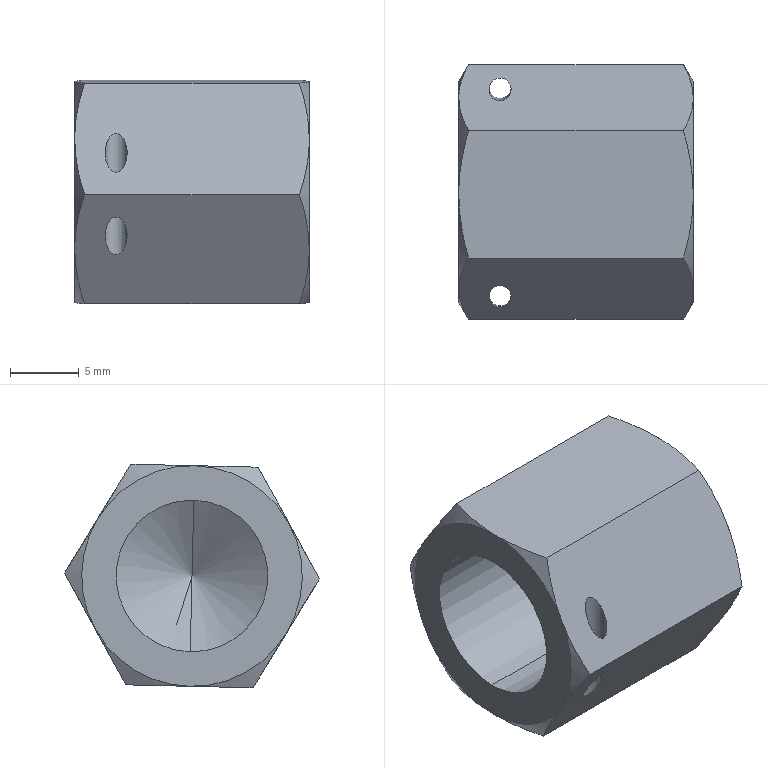Part | SolidWorks | features BaseBody 1 | 1 solid | 32 faces | box 17 x 18.47 x 16.209 mm | volume 2408 mm3 | cone 14 | plane 10 | cylinder 8 | commonest cylinder face diameters 1.6 x4 11 x2 12.5 x2
STEP:
#1=CARTESIAN_POINT('',(448.8,80.572,-3.182));
#2=VERTEX_POINT('',#1);
#3=CARTESIAN_POINT('',(450.4,80.572,-3.182));
#4=VERTEX_POINT('',#3);
#5=CARTESIAN_POINT('',(448.8,80.572,-3.182));
#6=CARTESIAN_POINT('',(448.8,78.908,-0.4485));
#7=CARTESIAN_POINT('',(450.4,78.908,-0.4485));
#8=CARTESIAN_POINT('',(450.4,80.572,-3.182));
#9=(BOUNDED_CURVE()B_SPLINE_CURVE(3,(#5,#6,#7,#8),.UNSPECIFIED.,.F.,.T.)B_SPLINE_CURVE_WITH_KNOTS((4,4),(4.712,7.854),.UNSPECIFIED.)CURVE()GEOMETRIC_REPRESENTATION_ITEM()RATIONAL_B_SPLINE_CURVE((1.,0.3333,0.3333,1.))REPRESENTATION_ITEM(''));
#10=EDGE_CURVE('',#2,#4,#9,.T.);
#11=ORIENTED_EDGE('',*,*,#10,.F.);
#12=CARTESIAN_POINT('',(448.8,80.432,2.836));
#13=VERTEX_POINT('',#12);
#14=CARTESIAN_POINT('',(448.8,80.687,-8.171));
#15=DIRECTION('',(0.,-0.0231,0.9997));
#16=VECTOR('',#15,1000.);
#17=LINE('',#14,#16);
#18=EDGE_CURVE('',#2,#13,#17,.T.);
#19=ORIENTED_EDGE('',*,*,#18,.T.);
#20=CARTESIAN_POINT('',(450.4,80.432,2.836));
#21=VERTEX_POINT('',#20);
#22=CARTESIAN_POINT('',(450.4,80.432,2.836));
#23=CARTESIAN_POINT('',(450.4,78.897,0.02809));
#24=CARTESIAN_POINT('',(448.8,78.897,0.02809));
#25=CARTESIAN_POINT('',(448.8,80.432,2.836));
#26=(BOUNDED_CURVE()B_SPLINE_CURVE(3,(#22,#23,#24,#25),.UNSPECIFIED.,.F.,.T.)B_SPLINE_CURVE_WITH_KNOTS((4,4),(1.571,4.712),.UNSPECIFIED.)CURVE()GEOMETRIC_REPRESENTATION_ITEM()RATIONAL_B_SPLINE_CURVE((1.,0.3333,0.3333,1.))REPRESENTATION_ITEM(''));
#27=EDGE_CURVE('',#21,#13,#26,.T.);
#28=ORIENTED_EDGE('',*,*,#27,.F.);
#29=CARTESIAN_POINT('',(450.4,80.687,-8.171));
#30=DIRECTION('',(0.,-0.0231,0.9997));
#31=VECTOR('',#30,1000.);
#32=LINE('',#29,#31);
#33=EDGE_CURVE('',#4,#21,#32,.T.);
#34=ORIENTED_EDGE('',*,*,#33,.F.);
#35=EDGE_LOOP('',(#11,#19,#28,#34));
#36=FACE_OUTER_BOUND('',#35,.T.);
#37=CARTESIAN_POINT('',(449.6,80.687,-8.171));
#38=DIRECTION('',(0.,-0.0231,0.9997));
#39=DIRECTION('',(1.,0.,0.));
#40=AXIS2_PLACEMENT_3D('',#37,#38,#39);
#41=CYLINDRICAL_SURFACE('',#40,0.8);
#42=ADVANCED_FACE('',(#36),#41,.F.);
#43=CARTESIAN_POINT('',(448.8,95.568,-2.836));
#44=VERTEX_POINT('',#43);
#45=CARTESIAN_POINT('',(450.4,95.568,-2.836));
#46=VERTEX_POINT('',#45);
#47=CARTESIAN_POINT('',(448.8,95.568,-2.836));
#48=CARTESIAN_POINT('',(448.8,94.032,-5.643));
#49=CARTESIAN_POINT('',(450.4,94.032,-5.643));
#50=CARTESIAN_POINT('',(450.4,95.568,-2.836));
#51=(BOUNDED_CURVE()B_SPLINE_CURVE(3,(#47,#48,#49,#50),.UNSPECIFIED.,.F.,.T.)B_SPLINE_CURVE_WITH_KNOTS((4,4),(1.571,4.712),.UNSPECIFIED.)CURVE()GEOMETRIC_REPRESENTATION_ITEM()RATIONAL_B_SPLINE_CURVE((1.,0.3333,0.3333,1.))REPRESENTATION_ITEM(''));
#52=EDGE_CURVE('',#44,#46,#51,.T.);
#53=ORIENTED_EDGE('',*,*,#52,.F.);
#54=CARTESIAN_POINT('',(448.8,95.428,3.182));
#55=VERTEX_POINT('',#54);
#56=CARTESIAN_POINT('',(448.8,95.683,-7.825));
#57=DIRECTION('',(0.,-0.0231,0.9997));
#58=VECTOR('',#57,1000.);
#59=LINE('',#56,#58);
#60=EDGE_CURVE('',#44,#55,#59,.T.);
#61=ORIENTED_EDGE('',*,*,#60,.T.);
#62=CARTESIAN_POINT('',(450.4,95.428,3.182));
#63=VERTEX_POINT('',#62);
#64=CARTESIAN_POINT('',(450.4,95.428,3.182));
#65=CARTESIAN_POINT('',(450.4,93.765,5.916));
#66=CARTESIAN_POINT('',(448.8,93.765,5.916));
#67=CARTESIAN_POINT('',(448.8,95.428,3.182));
#68=(BOUNDED_CURVE()B_SPLINE_CURVE(3,(#64,#65,#66,#67),.UNSPECIFIED.,.F.,.F.)B_SPLINE_CURVE_WITH_KNOTS((4,4),(4.712,7.854),.UNSPECIFIED.)CURVE()GEOMETRIC_REPRESENTATION_ITEM()RATIONAL_B_SPLINE_CURVE((1.,0.3333,0.3333,1.))REPRESENTATION_ITEM(''));
#69=EDGE_CURVE('',#63,#55,#68,.T.);
#70=ORIENTED_EDGE('',*,*,#69,.F.);
#71=CARTESIAN_POINT('',(450.4,95.683,-7.825));
#72=DIRECTION('',(0.,-0.0231,0.9997));
#73=VECTOR('',#72,1000.);
#74=LINE('',#71,#73);
#75=EDGE_CURVE('',#46,#63,#74,.T.);
#76=ORIENTED_EDGE('',*,*,#75,.F.);
#77=EDGE_LOOP('',(#53,#61,#70,#76));
#78=FACE_OUTER_BOUND('',#77,.T.);
#79=CARTESIAN_POINT('',(449.6,95.683,-7.825));
#80=DIRECTION('',(0.,-0.0231,0.9997));
#81=DIRECTION('',(1.,0.,0.));
#82=AXIS2_PLACEMENT_3D('',#79,#80,#81);
#83=CYLINDRICAL_SURFACE('',#82,0.8);
#84=ADVANCED_FACE('',(#78),#83,.F.);
#85=CARTESIAN_POINT('',(461.905,88.,0.));
#86=VERTEX_POINT('',#85);
#87=CARTESIAN_POINT('',(458.6,87.873,5.499));
#88=VERTEX_POINT('',#87);
#89=CARTESIAN_POINT('',(458.6,87.873,5.499));
#90=DIRECTION('',(-0.515,-0.0198,0.8569));
#91=VECTOR('',#90,1000.);
#92=LINE('',#89,#91);
#93=EDGE_CURVE('',#86,#88,#92,.T.);
#94=ORIENTED_EDGE('',*,*,#93,.F.);
#95=CARTESIAN_POINT('',(458.6,88.127,-5.499));
#96=VERTEX_POINT('',#95);
#97=CARTESIAN_POINT('',(458.6,88.127,-5.499));
#98=DIRECTION('',(-0.515,0.0198,-0.8569));
#99=VECTOR('',#98,1000.);
#100=LINE('',#97,#99);
#101=EDGE_CURVE('',#86,#96,#100,.T.);
#102=ORIENTED_EDGE('',*,*,#101,.T.);
#103=CARTESIAN_POINT('',(458.6,88.,0.));
#104=DIRECTION('',(-1.,0.,0.));
#105=DIRECTION('',(0.,-0.0231,0.9997));
#106=AXIS2_PLACEMENT_3D('',#103,#104,#105);
#107=CIRCLE('',#106,5.5);
#108=EDGE_CURVE('',#96,#88,#107,.T.);
#109=ORIENTED_EDGE('',*,*,#108,.T.);
#110=EDGE_LOOP('',(#94,#102,#109));
#111=FACE_OUTER_BOUND('',#110,.T.);
#112=CARTESIAN_POINT('',(458.6,88.,0.));
#113=DIRECTION('',(-1.,0.,0.));
#114=DIRECTION('',(0.,-0.0231,0.9997));
#115=AXIS2_PLACEMENT_3D('',#112,#113,#114);
#116=CONICAL_SURFACE('',#115,5.5,1.03);
#117=ADVANCED_FACE('',(#111),#116,.F.);
#118=CARTESIAN_POINT('',(455.6,88.144,-6.248));
#119=VERTEX_POINT('',#118);
#120=CARTESIAN_POINT('',(455.6,87.856,6.248));
#121=VERTEX_POINT('',#120);
#122=CARTESIAN_POINT('',(455.6,88.,0.));
#123=DIRECTION('',(-1.,0.,0.));
#124=DIRECTION('',(0.,-0.0231,0.9997));
#125=AXIS2_PLACEMENT_3D('',#122,#123,#124);
#126=CIRCLE('',#125,6.25);
#127=EDGE_CURVE('',#119,#121,#126,.T.);
#128=ORIENTED_EDGE('',*,*,#127,.T.);
#129=CARTESIAN_POINT('',(458.6,87.856,6.248));
#130=VERTEX_POINT('',#129);
#131=CARTESIAN_POINT('',(455.6,87.856,6.248));
#132=DIRECTION('',(1.,0.,0.));
#133=VECTOR('',#132,1000.);
#134=LINE('',#131,#133);
#135=EDGE_CURVE('',#121,#130,#134,.T.);
#136=ORIENTED_EDGE('',*,*,#135,.T.);
#137=CARTESIAN_POINT('',(458.6,88.144,-6.248));
#138=VERTEX_POINT('',#137);
#139=CARTESIAN_POINT('',(458.6,88.,0.));
#140=DIRECTION('',(-1.,0.,0.));
#141=DIRECTION('',(0.,-0.0231,0.9997));
#142=AXIS2_PLACEMENT_3D('',#139,#140,#141);
#143=CIRCLE('',#142,6.25);
#144=EDGE_CURVE('',#138,#130,#143,.T.);
#145=ORIENTED_EDGE('',*,*,#144,.F.);
#146=CARTESIAN_POINT('',(455.6,88.144,-6.248));
#147=DIRECTION('',(1.,0.,0.));
#148=VECTOR('',#147,1000.);
#149=LINE('',#146,#148);
#150=EDGE_CURVE('',#119,#138,#149,.T.);
#151=ORIENTED_EDGE('',*,*,#150,.F.);
#152=EDGE_LOOP('',(#128,#136,#145,#151));
#153=FACE_OUTER_BOUND('',#152,.T.);
#154=CARTESIAN_POINT('',(455.6,88.,0.));
#155=DIRECTION('',(1.,0.,0.));
#156=DIRECTION('',(0.,0.0231,-0.9997));
#157=AXIS2_PLACEMENT_3D('',#154,#155,#156);
#158=CYLINDRICAL_SURFACE('',#157,6.25);
#159=ADVANCED_FACE('',(#153),#158,.F.);
#160=CARTESIAN_POINT('',(455.6,87.873,5.499));
#161=VERTEX_POINT('',#160);
#162=CARTESIAN_POINT('',(455.6,88.127,-5.499));
#163=VERTEX_POINT('',#162);
#164=CARTESIAN_POINT('',(455.6,88.,0.));
#165=DIRECTION('',(1.,0.,0.));
#166=DIRECTION('',(0.,-0.0231,0.9997));
#167=AXIS2_PLACEMENT_3D('',#164,#165,#166);
#168=CIRCLE('',#167,5.5);
#169=EDGE_CURVE('',#161,#163,#168,.T.);
#170=ORIENTED_EDGE('',*,*,#169,.T.);
#171=CARTESIAN_POINT('',(446.6,88.127,-5.499));
#172=VERTEX_POINT('',#171);
#173=CARTESIAN_POINT('',(458.6,88.127,-5.499));
#174=DIRECTION('',(-1.,0.,0.));
#175=VECTOR('',#174,1000.);
#176=LINE('',#173,#175);
#177=EDGE_CURVE('',#163,#172,#176,.T.);
#178=ORIENTED_EDGE('',*,*,#177,.T.);
#179=CARTESIAN_POINT('',(446.6,87.873,5.499));
#180=VERTEX_POINT('',#179);
#181=CARTESIAN_POINT('',(446.6,88.,0.));
#182=DIRECTION('',(-1.,0.,0.));
#183=DIRECTION('',(0.,-0.0231,0.9997));
#184=AXIS2_PLACEMENT_3D('',#181,#182,#183);
#185=CIRCLE('',#184,5.5);
#186=EDGE_CURVE('',#172,#180,#185,.T.);
#187=ORIENTED_EDGE('',*,*,#186,.T.);
#188=CARTESIAN_POINT('',(458.6,87.873,5.499));
#189=DIRECTION('',(-1.,0.,0.));
#190=VECTOR('',#189,1000.);
#191=LINE('',#188,#190);
#192=EDGE_CURVE('',#161,#180,#191,.T.);
#193=ORIENTED_EDGE('',*,*,#192,.F.);
#194=EDGE_LOOP('',(#170,#178,#187,#193));
#195=FACE_OUTER_BOUND('',#194,.T.);
#196=CARTESIAN_POINT('',(458.6,88.,0.));
#197=DIRECTION('',(-1.,0.,0.));
#198=DIRECTION('',(0.,-0.0231,0.9997));
#199=AXIS2_PLACEMENT_3D('',#196,#197,#198);
#200=CYLINDRICAL_SURFACE('',#199,5.5);
#201=ADVANCED_FACE('',(#195),#200,.F.);
#202=ORIENTED_EDGE('',*,*,#69,.T.);
#203=CARTESIAN_POINT('',(448.8,95.428,3.182));
#204=CARTESIAN_POINT('',(448.8,97.092,0.4485));
#205=CARTESIAN_POINT('',(450.4,97.092,0.4485));
#206=CARTESIAN_POINT('',(450.4,95.428,3.182));
#207=(BOUNDED_CURVE()B_SPLINE_CURVE(3,(#203,#204,#205,#206),.UNSPECIFIED.,.F.,.T.)B_SPLINE_CURVE_WITH_KNOTS((4,4),(1.571,4.712),.UNSPECIFIED.)CURVE()GEOMETRIC_REPRESENTATION_ITEM()RATIONAL_B_SPLINE_CURVE((1.,0.3333,0.3333,1.))REPRESENTATION_ITEM(''));
#208=EDGE_CURVE('',#55,#63,#207,.T.);
#209=ORIENTED_EDGE('',*,*,#208,.T.);
#210=EDGE_LOOP('',(#202,#209));
#211=FACE_BOUND('',#210,.T.);
#212=CARTESIAN_POINT('',(462.885,97.235,0.2134));
#213=VERTEX_POINT('',#212);
#214=CARTESIAN_POINT('',(463.6,94.834,4.159));
#215=VERTEX_POINT('',#214);
#216=CARTESIAN_POINT('',(462.885,97.235,0.2134));
#217=CARTESIAN_POINT('',(463.102,96.845,0.8545));
#218=CARTESIAN_POINT('',(463.282,96.451,1.502));
#219=CARTESIAN_POINT('',(463.469,95.851,2.487));
#220=CARTESIAN_POINT('',(463.517,95.65,2.818));
#221=CARTESIAN_POINT('',(463.583,95.244,3.485));
#222=CARTESIAN_POINT('',(463.6,95.039,3.823));
#223=CARTESIAN_POINT('',(463.6,94.834,4.159));
#224=B_SPLINE_CURVE_WITH_KNOTS('',3,(#216,#217,#218,#219,#220,#221,#222,#223),.UNSPECIFIED.,.F.,.F.,(4,2,2,4),(0.001304,0.003639,0.004807,0.005975),.UNSPECIFIED.);
#225=EDGE_CURVE('',#213,#215,#224,.T.);
#226=ORIENTED_EDGE('',*,*,#225,.F.);
#227=CARTESIAN_POINT('',(447.315,97.235,0.2134));
#228=VERTEX_POINT('',#227);
#229=CARTESIAN_POINT('',(446.6,97.235,0.2134));
#230=DIRECTION('',(1.,0.,0.));
#231=VECTOR('',#230,1000.);
#232=LINE('',#229,#231);
#233=EDGE_CURVE('',#228,#213,#232,.T.);
#234=ORIENTED_EDGE('',*,*,#233,.F.);
#235=CARTESIAN_POINT('',(446.6,94.834,4.159));
#236=VERTEX_POINT('',#235);
#237=CARTESIAN_POINT('',(446.6,94.834,4.159));
#238=CARTESIAN_POINT('',(446.6,95.039,3.823));
#239=CARTESIAN_POINT('',(446.617,95.244,3.485));
#240=CARTESIAN_POINT('',(446.683,95.65,2.818));
#241=CARTESIAN_POINT('',(446.731,95.851,2.487));
#242=CARTESIAN_POINT('',(446.918,96.451,1.502));
#243=CARTESIAN_POINT('',(447.098,96.845,0.8545));
#244=CARTESIAN_POINT('',(447.315,97.235,0.2134));
#245=B_SPLINE_CURVE_WITH_KNOTS('',3,(#237,#238,#239,#240,#241,#242,#243,#244),.UNSPECIFIED.,.F.,.F.,(4,2,2,4),(0.005009,0.006177,0.007344,0.009679),.UNSPECIFIED.);
#246=EDGE_CURVE('',#236,#228,#245,.T.);
#247=ORIENTED_EDGE('',*,*,#246,.F.);
#248=CARTESIAN_POINT('',(447.315,92.433,8.105));
#249=VERTEX_POINT('',#248);
#250=CARTESIAN_POINT('',(447.315,92.433,8.105));
#251=CARTESIAN_POINT('',(447.097,92.825,7.46));
#252=CARTESIAN_POINT('',(446.917,93.22,6.81));
#253=CARTESIAN_POINT('',(446.668,94.02,5.496));
#254=CARTESIAN_POINT('',(446.6,94.424,4.832));
#255=CARTESIAN_POINT('',(446.6,94.834,4.159));
#256=B_SPLINE_CURVE_WITH_KNOTS('',3,(#250,#251,#252,#253,#254,#255),.UNSPECIFIED.,.F.,.F.,(4,2,4),(0.0003354,0.002672,0.005009),.UNSPECIFIED.);
#257=EDGE_CURVE('',#249,#236,#256,.T.);
#258=ORIENTED_EDGE('',*,*,#257,.F.);
#259=CARTESIAN_POINT('',(462.885,92.433,8.105));
#260=VERTEX_POINT('',#259);
#261=CARTESIAN_POINT('',(446.6,92.433,8.105));
#262=DIRECTION('',(1.,0.,0.));
#263=VECTOR('',#262,1000.);
#264=LINE('',#261,#263);
#265=EDGE_CURVE('',#249,#260,#264,.T.);
#266=ORIENTED_EDGE('',*,*,#265,.T.);
#267=CARTESIAN_POINT('',(463.6,94.834,4.159));
#268=CARTESIAN_POINT('',(463.6,94.424,4.832));
#269=CARTESIAN_POINT('',(463.532,94.02,5.496));
#270=CARTESIAN_POINT('',(463.283,93.22,6.81));
#271=CARTESIAN_POINT('',(463.103,92.825,7.46));
#272=CARTESIAN_POINT('',(462.885,92.433,8.105));
#273=B_SPLINE_CURVE_WITH_KNOTS('',3,(#267,#268,#269,#270,#271,#272),.UNSPECIFIED.,.F.,.F.,(4,2,4),(0.005975,0.008312,0.01065),.UNSPECIFIED.);
#274=EDGE_CURVE('',#215,#260,#273,.T.);
#275=ORIENTED_EDGE('',*,*,#274,.F.);
#276=EDGE_LOOP('',(#226,#234,#247,#258,#266,#275));
#277=FACE_OUTER_BOUND('',#276,.T.);
#278=CARTESIAN_POINT('',(446.6,92.433,8.105));
#279=DIRECTION('',(0.,-0.8542,-0.5199));
#280=DIRECTION('',(0.,-0.5199,0.8542));
#281=AXIS2_PLACEMENT_3D('',#278,#279,#280);
#282=PLANE('',#281);
#283=ADVANCED_FACE('',(#211,#277),#282,.F.);
#284=CARTESIAN_POINT('',(450.4,95.568,-2.836));
#285=CARTESIAN_POINT('',(450.4,97.103,-0.02809));
#286=CARTESIAN_POINT('',(448.8,97.103,-0.02809));
#287=CARTESIAN_POINT('',(448.8,95.568,-2.836));
#288=(BOUNDED_CURVE()B_SPLINE_CURVE(3,(#284,#285,#286,#287),.UNSPECIFIED.,.F.,.F.)B_SPLINE_CURVE_WITH_KNOTS((4,4),(4.712,7.854),.UNSPECIFIED.)CURVE()GEOMETRIC_REPRESENTATION_ITEM()RATIONAL_B_SPLINE_CURVE((1.,0.3333,0.3333,1.))REPRESENTATION_ITEM(''));
#289=EDGE_CURVE('',#46,#44,#288,.T.);
#290=ORIENTED_EDGE('',*,*,#289,.T.);
#291=ORIENTED_EDGE('',*,*,#52,.T.);
#292=EDGE_LOOP('',(#290,#291));
#293=FACE_BOUND('',#292,.T.);
#294=CARTESIAN_POINT('',(462.885,92.802,-7.891));
#295=VERTEX_POINT('',#294);
#296=CARTESIAN_POINT('',(463.6,95.019,-3.839));
#297=VERTEX_POINT('',#296);
#298=CARTESIAN_POINT('',(462.885,92.802,-7.891));
#299=CARTESIAN_POINT('',(463.102,93.163,-7.232));
#300=CARTESIAN_POINT('',(463.284,93.532,-6.557));
#301=CARTESIAN_POINT('',(463.533,94.272,-5.204));
#302=CARTESIAN_POINT('',(463.6,94.644,-4.524));
#303=CARTESIAN_POINT('',(463.6,95.019,-3.839));
#304=B_SPLINE_CURVE_WITH_KNOTS('',3,(#298,#299,#300,#301,#302,#303),.UNSPECIFIED.,.F.,.F.,(4,2,4),(0.008227,0.01056,0.0129),.UNSPECIFIED.);
#305=EDGE_CURVE('',#295,#297,#304,.T.);
#306=ORIENTED_EDGE('',*,*,#305,.F.);
#307=CARTESIAN_POINT('',(447.315,92.802,-7.891));
#308=VERTEX_POINT('',#307);
#309=CARTESIAN_POINT('',(446.6,92.802,-7.891));
#310=DIRECTION('',(1.,0.,0.));
#311=VECTOR('',#310,1000.);
#312=LINE('',#309,#311);
#313=EDGE_CURVE('',#308,#295,#312,.T.);
#314=ORIENTED_EDGE('',*,*,#313,.F.);
#315=CARTESIAN_POINT('',(446.6,95.019,-3.839));
#316=VERTEX_POINT('',#315);
#317=CARTESIAN_POINT('',(446.6,95.019,-3.839));
#318=CARTESIAN_POINT('',(446.6,94.644,-4.524));
#319=CARTESIAN_POINT('',(446.667,94.272,-5.204));
#320=CARTESIAN_POINT('',(446.916,93.532,-6.557));
#321=CARTESIAN_POINT('',(447.098,93.163,-7.232));
#322=CARTESIAN_POINT('',(447.315,92.802,-7.891));
#323=B_SPLINE_CURVE_WITH_KNOTS('',3,(#317,#318,#319,#320,#321,#322),.UNSPECIFIED.,.F.,.F.,(4,2,4),(0.008064,0.01039,0.01272),.UNSPECIFIED.);
#324=EDGE_CURVE('',#316,#308,#323,.T.);
#325=ORIENTED_EDGE('',*,*,#324,.F.);
#326=CARTESIAN_POINT('',(447.315,97.235,0.2134));
#327=CARTESIAN_POINT('',(447.099,96.877,-0.4419));
#328=CARTESIAN_POINT('',(446.919,96.514,-1.106));
#329=CARTESIAN_POINT('',(446.669,95.773,-2.459));
#330=CARTESIAN_POINT('',(446.6,95.393,-3.154));
#331=CARTESIAN_POINT('',(446.6,95.019,-3.839));
#332=B_SPLINE_CURVE_WITH_KNOTS('',3,(#326,#327,#328,#329,#330,#331),.UNSPECIFIED.,.F.,.F.,(4,2,4),(0.003401,0.005732,0.008064),.UNSPECIFIED.);
#333=EDGE_CURVE('',#228,#316,#332,.T.);
#334=ORIENTED_EDGE('',*,*,#333,.F.);
#335=ORIENTED_EDGE('',*,*,#233,.T.);
#336=CARTESIAN_POINT('',(463.6,95.019,-3.839));
#337=CARTESIAN_POINT('',(463.6,95.393,-3.154));
#338=CARTESIAN_POINT('',(463.531,95.773,-2.459));
#339=CARTESIAN_POINT('',(463.281,96.514,-1.106));
#340=CARTESIAN_POINT('',(463.101,96.877,-0.4419));
#341=CARTESIAN_POINT('',(462.885,97.235,0.2134));
#342=B_SPLINE_CURVE_WITH_KNOTS('',3,(#336,#337,#338,#339,#340,#341),.UNSPECIFIED.,.F.,.F.,(4,2,4),(0.0129,0.01524,0.01757),.UNSPECIFIED.);
#343=EDGE_CURVE('',#297,#213,#342,.T.);
#344=ORIENTED_EDGE('',*,*,#343,.F.);
#345=EDGE_LOOP('',(#306,#314,#325,#334,#335,#344));
#346=FACE_OUTER_BOUND('',#345,.T.);
#347=CARTESIAN_POINT('',(446.6,97.235,0.2134));
#348=DIRECTION('',(0.,-0.8773,0.4799));
#349=DIRECTION('',(0.,0.4799,0.8773));
#350=AXIS2_PLACEMENT_3D('',#347,#348,#349);
#351=PLANE('',#350);
#352=ADVANCED_FACE('',(#293,#346),#351,.F.);
#353=CARTESIAN_POINT('',(462.885,83.567,-8.105));
#354=VERTEX_POINT('',#353);
#355=CARTESIAN_POINT('',(463.6,88.185,-7.998));
#356=VERTEX_POINT('',#355);
#357=CARTESIAN_POINT('',(462.885,83.567,-8.105));
#358=CARTESIAN_POINT('',(463.103,84.319,-8.087));
#359=CARTESIAN_POINT('',(463.284,85.088,-8.069));
#360=CARTESIAN_POINT('',(463.533,86.628,-8.034));
#361=CARTESIAN_POINT('',(463.6,87.403,-8.016));
#362=CARTESIAN_POINT('',(463.6,88.185,-7.998));
#363=B_SPLINE_CURVE_WITH_KNOTS('',3,(#357,#358,#359,#360,#361,#362),.UNSPECIFIED.,.F.,.F.,(4,2,4),(0.008667,0.01101,0.01334),.UNSPECIFIED.);
#364=EDGE_CURVE('',#354,#356,#363,.T.);
#365=ORIENTED_EDGE('',*,*,#364,.F.);
#366=CARTESIAN_POINT('',(447.315,83.567,-8.105));
#367=VERTEX_POINT('',#366);
#368=CARTESIAN_POINT('',(446.6,83.567,-8.105));
#369=DIRECTION('',(1.,0.,0.));
#370=VECTOR('',#369,1000.);
#371=LINE('',#368,#370);
#372=EDGE_CURVE('',#367,#354,#371,.T.);
#373=ORIENTED_EDGE('',*,*,#372,.F.);
#374=CARTESIAN_POINT('',(446.6,88.185,-7.998));
#375=VERTEX_POINT('',#374);
#376=CARTESIAN_POINT('',(446.6,88.185,-7.998));
#377=CARTESIAN_POINT('',(446.6,87.403,-8.016));
#378=CARTESIAN_POINT('',(446.667,86.628,-8.034));
#379=CARTESIAN_POINT('',(446.916,85.088,-8.069));
#380=CARTESIAN_POINT('',(447.097,84.319,-8.087));
#381=CARTESIAN_POINT('',(447.315,83.567,-8.105));
#382=B_SPLINE_CURVE_WITH_KNOTS('',3,(#376,#377,#378,#379,#380,#381),.UNSPECIFIED.,.F.,.F.,(4,2,4),(0.03992,0.04226,0.04459),.UNSPECIFIED.);
#383=EDGE_CURVE('',#375,#367,#382,.T.);
#384=ORIENTED_EDGE('',*,*,#383,.F.);
#385=CARTESIAN_POINT('',(447.315,92.802,-7.891));
#386=CARTESIAN_POINT('',(447.099,92.055,-7.908));
#387=CARTESIAN_POINT('',(446.919,91.299,-7.926));
#388=CARTESIAN_POINT('',(446.732,90.144,-7.953));
#389=CARTESIAN_POINT('',(446.683,89.755,-7.962));
#390=CARTESIAN_POINT('',(446.617,88.97,-7.98));
#391=CARTESIAN_POINT('',(446.6,88.576,-7.989));
#392=CARTESIAN_POINT('',(446.6,88.185,-7.998));
#393=B_SPLINE_CURVE_WITH_KNOTS('',3,(#385,#386,#387,#388,#389,#390,#391,#392),.UNSPECIFIED.,.F.,.F.,(4,2,2,4),(0.03525,0.03759,0.03875,0.03992),.UNSPECIFIED.);
#394=EDGE_CURVE('',#308,#375,#393,.T.);
#395=ORIENTED_EDGE('',*,*,#394,.F.);
#396=ORIENTED_EDGE('',*,*,#313,.T.);
#397=CARTESIAN_POINT('',(463.6,88.185,-7.998));
#398=CARTESIAN_POINT('',(463.6,88.576,-7.989));
#399=CARTESIAN_POINT('',(463.583,88.97,-7.98));
#400=CARTESIAN_POINT('',(463.517,89.755,-7.962));
#401=CARTESIAN_POINT('',(463.468,90.144,-7.953));
#402=CARTESIAN_POINT('',(463.281,91.299,-7.926));
#403=CARTESIAN_POINT('',(463.101,92.055,-7.908));
#404=CARTESIAN_POINT('',(462.885,92.802,-7.891));
#405=B_SPLINE_CURVE_WITH_KNOTS('',3,(#397,#398,#399,#400,#401,#402,#403,#404),.UNSPECIFIED.,.F.,.F.,(4,2,2,4),(0.01334,0.01451,0.01568,0.01802),.UNSPECIFIED.);
#406=EDGE_CURVE('',#356,#295,#405,.T.);
#407=ORIENTED_EDGE('',*,*,#406,.F.);
#408=EDGE_LOOP('',(#365,#373,#384,#395,#396,#407));
#409=FACE_OUTER_BOUND('',#408,.T.);
#410=CARTESIAN_POINT('',(446.6,92.802,-7.891));
#411=DIRECTION('',(0.,-0.0231,0.9997));
#412=DIRECTION('',(1.,0.,0.));
#413=AXIS2_PLACEMENT_3D('',#410,#411,#412);
#414=PLANE('',#413);
#415=ADVANCED_FACE('',(#409),#414,.F.);
#416=CARTESIAN_POINT('',(450.4,80.572,-3.182));
#417=CARTESIAN_POINT('',(450.4,82.235,-5.916));
#418=CARTESIAN_POINT('',(448.8,82.235,-5.916));
#419=CARTESIAN_POINT('',(448.8,80.572,-3.182));
#420=(BOUNDED_CURVE()B_SPLINE_CURVE(3,(#416,#417,#418,#419),.UNSPECIFIED.,.F.,.F.)B_SPLINE_CURVE_WITH_KNOTS((4,4),(1.571,4.712),.UNSPECIFIED.)CURVE()GEOMETRIC_REPRESENTATION_ITEM()RATIONAL_B_SPLINE_CURVE((1.,0.3333,0.3333,1.))REPRESENTATION_ITEM(''));
#421=EDGE_CURVE('',#4,#2,#420,.T.);
#422=ORIENTED_EDGE('',*,*,#421,.T.);
#423=ORIENTED_EDGE('',*,*,#10,.T.);
#424=EDGE_LOOP('',(#422,#423));
#425=FACE_BOUND('',#424,.T.);
#426=CARTESIAN_POINT('',(462.885,78.765,-0.2134));
#427=VERTEX_POINT('',#426);
#428=CARTESIAN_POINT('',(463.6,81.166,-4.159));
#429=VERTEX_POINT('',#428);
#430=CARTESIAN_POINT('',(462.885,78.765,-0.2134));
#431=CARTESIAN_POINT('',(462.993,78.959,-0.5324));
#432=CARTESIAN_POINT('',(463.092,79.155,-0.8547));
#433=CARTESIAN_POINT('',(463.269,79.552,-1.508));
#434=CARTESIAN_POINT('',(463.346,79.754,-1.838));
#435=CARTESIAN_POINT('',(463.533,80.356,-2.828));
#436=CARTESIAN_POINT('',(463.6,80.76,-3.492));
#437=CARTESIAN_POINT('',(463.6,81.166,-4.159));
#438=B_SPLINE_CURVE_WITH_KNOTS('',3,(#430,#431,#432,#433,#434,#435,#436,#437),.UNSPECIFIED.,.F.,.F.,(4,2,2,4),(0.01545,0.01661,0.01776,0.02008),.UNSPECIFIED.);
#439=EDGE_CURVE('',#427,#429,#438,.T.);
#440=ORIENTED_EDGE('',*,*,#439,.F.);
#441=CARTESIAN_POINT('',(447.315,78.765,-0.2134));
#442=VERTEX_POINT('',#441);
#443=CARTESIAN_POINT('',(446.6,78.765,-0.2134));
#444=DIRECTION('',(1.,0.,0.));
#445=VECTOR('',#444,1000.);
#446=LINE('',#443,#445);
#447=EDGE_CURVE('',#442,#427,#446,.T.);
#448=ORIENTED_EDGE('',*,*,#447,.F.);
#449=CARTESIAN_POINT('',(446.6,81.166,-4.159));
#450=VERTEX_POINT('',#449);
#451=CARTESIAN_POINT('',(446.6,81.166,-4.159));
#452=CARTESIAN_POINT('',(446.6,80.76,-3.492));
#453=CARTESIAN_POINT('',(446.667,80.356,-2.828));
#454=CARTESIAN_POINT('',(446.854,79.754,-1.838));
#455=CARTESIAN_POINT('',(446.931,79.552,-1.508));
#456=CARTESIAN_POINT('',(447.108,79.155,-0.8547));
#457=CARTESIAN_POINT('',(447.207,78.959,-0.5324));
#458=CARTESIAN_POINT('',(447.315,78.765,-0.2134));
#459=B_SPLINE_CURVE_WITH_KNOTS('',3,(#451,#452,#453,#454,#455,#456,#457,#458),.UNSPECIFIED.,.F.,.F.,(4,2,2,4),(0.007717,0.01005,0.01121,0.01238),.UNSPECIFIED.);
#460=EDGE_CURVE('',#450,#442,#459,.T.);
#461=ORIENTED_EDGE('',*,*,#460,.F.);
#462=CARTESIAN_POINT('',(447.315,83.567,-8.105));
#463=CARTESIAN_POINT('',(447.099,83.179,-7.466));
#464=CARTESIAN_POINT('',(446.919,82.785,-6.82));
#465=CARTESIAN_POINT('',(446.669,81.983,-5.502));
#466=CARTESIAN_POINT('',(446.6,81.572,-4.826));
#467=CARTESIAN_POINT('',(446.6,81.166,-4.159));
#468=B_SPLINE_CURVE_WITH_KNOTS('',3,(#462,#463,#464,#465,#466,#467),.UNSPECIFIED.,.F.,.F.,(4,2,4),(0.003051,0.005384,0.007717),.UNSPECIFIED.);
#469=EDGE_CURVE('',#367,#450,#468,.T.);
#470=ORIENTED_EDGE('',*,*,#469,.F.);
#471=ORIENTED_EDGE('',*,*,#372,.T.);
#472=CARTESIAN_POINT('',(463.6,81.166,-4.159));
#473=CARTESIAN_POINT('',(463.6,81.572,-4.826));
#474=CARTESIAN_POINT('',(463.531,81.983,-5.502));
#475=CARTESIAN_POINT('',(463.281,82.785,-6.82));
#476=CARTESIAN_POINT('',(463.101,83.179,-7.466));
#477=CARTESIAN_POINT('',(462.885,83.567,-8.105));
#478=B_SPLINE_CURVE_WITH_KNOTS('',3,(#472,#473,#474,#475,#476,#477),.UNSPECIFIED.,.F.,.F.,(4,2,4),(0.02008,0.02239,0.0247),.UNSPECIFIED.);
#479=EDGE_CURVE('',#429,#354,#478,.T.);
#480=ORIENTED_EDGE('',*,*,#479,.F.);
#481=EDGE_LOOP('',(#440,#448,#461,#470,#471,#480));
#482=FACE_OUTER_BOUND('',#481,.T.);
#483=CARTESIAN_POINT('',(446.6,83.567,-8.105));
#484=DIRECTION('',(0.,0.8542,0.5199));
#485=DIRECTION('',(0.,0.5199,-0.8542));
#486=AXIS2_PLACEMENT_3D('',#483,#484,#485);
#487=PLANE('',#486);
#488=ADVANCED_FACE('',(#425,#482),#487,.F.);
#489=ORIENTED_EDGE('',*,*,#27,.T.);
#490=CARTESIAN_POINT('',(448.8,80.432,2.836));
#491=CARTESIAN_POINT('',(448.8,81.968,5.643));
#492=CARTESIAN_POINT('',(450.4,81.968,5.643));
#493=CARTESIAN_POINT('',(450.4,80.432,2.836));
#494=(BOUNDED_CURVE()B_SPLINE_CURVE(3,(#490,#491,#492,#493),.UNSPECIFIED.,.F.,.F.)B_SPLINE_CURVE_WITH_KNOTS((4,4),(4.712,7.854),.UNSPECIFIED.)CURVE()GEOMETRIC_REPRESENTATION_ITEM()RATIONAL_B_SPLINE_CURVE((1.,0.3333,0.3333,1.))REPRESENTATION_ITEM(''));
#495=EDGE_CURVE('',#13,#21,#494,.T.);
#496=ORIENTED_EDGE('',*,*,#495,.T.);
#497=EDGE_LOOP('',(#489,#496));
#498=FACE_BOUND('',#497,.T.);
#499=CARTESIAN_POINT('',(462.885,83.198,7.891));
#500=VERTEX_POINT('',#499);
#501=CARTESIAN_POINT('',(463.6,80.981,3.839));
#502=VERTEX_POINT('',#501);
#503=CARTESIAN_POINT('',(462.885,83.198,7.891));
#504=CARTESIAN_POINT('',(463.101,82.839,7.236));
#505=CARTESIAN_POINT('',(463.281,82.476,6.572));
#506=CARTESIAN_POINT('',(463.531,81.736,5.219));
#507=CARTESIAN_POINT('',(463.6,81.356,4.524));
#508=CARTESIAN_POINT('',(463.6,80.981,3.839));
#509=B_SPLINE_CURVE_WITH_KNOTS('',3,(#503,#504,#505,#506,#507,#508),.UNSPECIFIED.,.F.,.F.,(4,2,4),(0.003357,0.005689,0.00802),.UNSPECIFIED.);
#510=EDGE_CURVE('',#500,#502,#509,.T.);
#511=ORIENTED_EDGE('',*,*,#510,.F.);
#512=CARTESIAN_POINT('',(447.315,83.198,7.891));
#513=VERTEX_POINT('',#512);
#514=CARTESIAN_POINT('',(446.6,83.198,7.891));
#515=DIRECTION('',(1.,0.,0.));
#516=VECTOR('',#515,1000.);
#517=LINE('',#514,#516);
#518=EDGE_CURVE('',#513,#500,#517,.T.);
#519=ORIENTED_EDGE('',*,*,#518,.F.);
#520=CARTESIAN_POINT('',(446.6,80.981,3.839));
#521=VERTEX_POINT('',#520);
#522=CARTESIAN_POINT('',(446.6,80.981,3.839));
#523=CARTESIAN_POINT('',(446.6,81.356,4.524));
#524=CARTESIAN_POINT('',(446.669,81.736,5.219));
#525=CARTESIAN_POINT('',(446.919,82.476,6.572));
#526=CARTESIAN_POINT('',(447.099,82.839,7.236));
#527=CARTESIAN_POINT('',(447.315,83.198,7.891));
#528=B_SPLINE_CURVE_WITH_KNOTS('',3,(#522,#523,#524,#525,#526,#527),.UNSPECIFIED.,.F.,.F.,(4,2,4),(0.01294,0.01528,0.01762),.UNSPECIFIED.);
#529=EDGE_CURVE('',#521,#513,#528,.T.);
#530=ORIENTED_EDGE('',*,*,#529,.F.);
#531=CARTESIAN_POINT('',(447.315,78.765,-0.2134));
#532=CARTESIAN_POINT('',(447.098,79.125,0.4458));
#533=CARTESIAN_POINT('',(446.916,79.495,1.121));
#534=CARTESIAN_POINT('',(446.667,80.235,2.474));
#535=CARTESIAN_POINT('',(446.6,80.607,3.154));
#536=CARTESIAN_POINT('',(446.6,80.981,3.839));
#537=B_SPLINE_CURVE_WITH_KNOTS('',3,(#531,#532,#533,#534,#535,#536),.UNSPECIFIED.,.F.,.F.,(4,2,4),(0.008267,0.0106,0.01294),.UNSPECIFIED.);
#538=EDGE_CURVE('',#442,#521,#537,.T.);
#539=ORIENTED_EDGE('',*,*,#538,.F.);
#540=ORIENTED_EDGE('',*,*,#447,.T.);
#541=CARTESIAN_POINT('',(463.6,80.981,3.839));
#542=CARTESIAN_POINT('',(463.6,80.607,3.154));
#543=CARTESIAN_POINT('',(463.533,80.235,2.474));
#544=CARTESIAN_POINT('',(463.284,79.495,1.121));
#545=CARTESIAN_POINT('',(463.102,79.125,0.4458));
#546=CARTESIAN_POINT('',(462.885,78.765,-0.2134));
#547=B_SPLINE_CURVE_WITH_KNOTS('',3,(#541,#542,#543,#544,#545,#546),.UNSPECIFIED.,.F.,.F.,(4,2,4),(0.00802,0.01035,0.01268),.UNSPECIFIED.);
#548=EDGE_CURVE('',#502,#427,#547,.T.);
#549=ORIENTED_EDGE('',*,*,#548,.F.);
#550=EDGE_LOOP('',(#511,#519,#530,#539,#540,#549));
#551=FACE_OUTER_BOUND('',#550,.T.);
#552=CARTESIAN_POINT('',(446.6,78.765,-0.2134));
#553=DIRECTION('',(0.,0.8773,-0.4799));
#554=DIRECTION('',(0.,-0.4799,-0.8773));
#555=AXIS2_PLACEMENT_3D('',#552,#553,#554);
#556=PLANE('',#555);
#557=ADVANCED_FACE('',(#498,#551),#556,.F.);
#558=CARTESIAN_POINT('',(463.6,87.815,7.998));
#559=VERTEX_POINT('',#558);
#560=CARTESIAN_POINT('',(462.885,92.433,8.105));
#561=CARTESIAN_POINT('',(463.101,91.686,8.087));
#562=CARTESIAN_POINT('',(463.281,90.93,8.07));
#563=CARTESIAN_POINT('',(463.468,89.774,8.043));
#564=CARTESIAN_POINT('',(463.517,89.386,8.034));
#565=CARTESIAN_POINT('',(463.583,88.6,8.016));
#566=CARTESIAN_POINT('',(463.6,88.206,8.007));
#567=CARTESIAN_POINT('',(463.6,87.815,7.998));
#568=B_SPLINE_CURVE_WITH_KNOTS('',3,(#560,#561,#562,#563,#564,#565,#566,#567),.UNSPECIFIED.,.F.,.F.,(4,2,2,4),(0.03525,0.03759,0.03875,0.03992),.UNSPECIFIED.);
#569=EDGE_CURVE('',#260,#559,#568,.T.);
#570=ORIENTED_EDGE('',*,*,#569,.F.);
#571=ORIENTED_EDGE('',*,*,#265,.F.);
#572=CARTESIAN_POINT('',(446.6,87.815,7.998));
#573=VERTEX_POINT('',#572);
#574=CARTESIAN_POINT('',(446.6,87.815,7.998));
#575=CARTESIAN_POINT('',(446.6,88.206,8.007));
#576=CARTESIAN_POINT('',(446.617,88.6,8.016));
#577=CARTESIAN_POINT('',(446.683,89.386,8.034));
#578=CARTESIAN_POINT('',(446.732,89.774,8.043));
#579=CARTESIAN_POINT('',(446.919,90.93,8.07));
#580=CARTESIAN_POINT('',(447.099,91.686,8.087));
#581=CARTESIAN_POINT('',(447.315,92.433,8.105));
#582=B_SPLINE_CURVE_WITH_KNOTS('',3,(#574,#575,#576,#577,#578,#579,#580,#581),.UNSPECIFIED.,.F.,.F.,(4,2,2,4),(0.01334,0.01451,0.01568,0.01802),.UNSPECIFIED.);
#583=EDGE_CURVE('',#573,#249,#582,.T.);
#584=ORIENTED_EDGE('',*,*,#583,.F.);
#585=CARTESIAN_POINT('',(447.315,83.198,7.891));
#586=CARTESIAN_POINT('',(447.097,83.95,7.909));
#587=CARTESIAN_POINT('',(446.916,84.718,7.926));
#588=CARTESIAN_POINT('',(446.667,86.258,7.962));
#589=CARTESIAN_POINT('',(446.6,87.034,7.98));
#590=CARTESIAN_POINT('',(446.6,87.815,7.998));
#591=B_SPLINE_CURVE_WITH_KNOTS('',3,(#585,#586,#587,#588,#589,#590),.UNSPECIFIED.,.F.,.F.,(4,2,4),(0.008667,0.01101,0.01334),.UNSPECIFIED.);
#592=EDGE_CURVE('',#513,#573,#591,.T.);
#593=ORIENTED_EDGE('',*,*,#592,.F.);
#594=ORIENTED_EDGE('',*,*,#518,.T.);
#595=CARTESIAN_POINT('',(463.6,87.815,7.998));
#596=CARTESIAN_POINT('',(463.6,87.034,7.98));
#597=CARTESIAN_POINT('',(463.533,86.258,7.962));
#598=CARTESIAN_POINT('',(463.284,84.718,7.926));
#599=CARTESIAN_POINT('',(463.103,83.95,7.909));
#600=CARTESIAN_POINT('',(462.885,83.198,7.891));
#601=B_SPLINE_CURVE_WITH_KNOTS('',3,(#595,#596,#597,#598,#599,#600),.UNSPECIFIED.,.F.,.F.,(4,2,4),(0.03992,0.04226,0.04459),.UNSPECIFIED.);
#602=EDGE_CURVE('',#559,#500,#601,.T.);
#603=ORIENTED_EDGE('',*,*,#602,.F.);
#604=EDGE_LOOP('',(#570,#571,#584,#593,#594,#603));
#605=FACE_OUTER_BOUND('',#604,.T.);
#606=CARTESIAN_POINT('',(446.6,83.198,7.891));
#607=DIRECTION('',(0.,0.0231,-0.9997));
#608=DIRECTION('',(-1.,0.,0.));
#609=AXIS2_PLACEMENT_3D('',#606,#607,#608);
#610=PLANE('',#609);
#611=ADVANCED_FACE('',(#605),#610,.F.);
#612=ORIENTED_EDGE('',*,*,#529,.T.);
#613=ORIENTED_EDGE('',*,*,#592,.T.);
#614=CARTESIAN_POINT('',(446.6,88.,0.));
#615=DIRECTION('',(-1.,0.,0.));
#616=DIRECTION('',(0.,-0.0231,0.9997));
#617=AXIS2_PLACEMENT_3D('',#614,#615,#616);
#618=CIRCLE('',#617,8.);
#619=EDGE_CURVE('',#521,#573,#618,.T.);
#620=ORIENTED_EDGE('',*,*,#619,.F.);
#621=EDGE_LOOP('',(#612,#613,#620));
#622=FACE_OUTER_BOUND('',#621,.T.);
#623=CARTESIAN_POINT('',(446.6,88.,0.));
#624=DIRECTION('',(1.,0.,0.));
#625=DIRECTION('',(0.,-0.0231,0.9997));
#626=AXIS2_PLACEMENT_3D('',#623,#624,#625);
#627=CONICAL_SURFACE('',#626,8.,1.047);
#628=ADVANCED_FACE('',(#622),#627,.T.);
#629=ORIENTED_EDGE('',*,*,#460,.T.);
#630=ORIENTED_EDGE('',*,*,#538,.T.);
#631=CARTESIAN_POINT('',(446.6,88.,0.));
#632=DIRECTION('',(-1.,0.,0.));
#633=DIRECTION('',(0.,-0.0231,0.9997));
#634=AXIS2_PLACEMENT_3D('',#631,#632,#633);
#635=CIRCLE('',#634,8.);
#636=EDGE_CURVE('',#450,#521,#635,.T.);
#637=ORIENTED_EDGE('',*,*,#636,.F.);
#638=EDGE_LOOP('',(#629,#630,#637));
#639=FACE_OUTER_BOUND('',#638,.T.);
#640=CARTESIAN_POINT('',(446.6,88.,0.));
#641=DIRECTION('',(1.,0.,0.));
#642=DIRECTION('',(0.,-0.0231,0.9997));
#643=AXIS2_PLACEMENT_3D('',#640,#641,#642);
#644=CONICAL_SURFACE('',#643,8.,1.047);
#645=ADVANCED_FACE('',(#639),#644,.T.);
#646=ORIENTED_EDGE('',*,*,#383,.T.);
#647=ORIENTED_EDGE('',*,*,#469,.T.);
#648=CARTESIAN_POINT('',(446.6,88.,0.));
#649=DIRECTION('',(-1.,0.,0.));
#650=DIRECTION('',(0.,-0.0231,0.9997));
#651=AXIS2_PLACEMENT_3D('',#648,#649,#650);
#652=CIRCLE('',#651,8.);
#653=EDGE_CURVE('',#375,#450,#652,.T.);
#654=ORIENTED_EDGE('',*,*,#653,.F.);
#655=EDGE_LOOP('',(#646,#647,#654));
#656=FACE_OUTER_BOUND('',#655,.T.);
#657=CARTESIAN_POINT('',(446.6,88.,0.));
#658=DIRECTION('',(1.,0.,0.));
#659=DIRECTION('',(0.,-0.0231,0.9997));
#660=AXIS2_PLACEMENT_3D('',#657,#658,#659);
#661=CONICAL_SURFACE('',#660,8.,1.047);
#662=ADVANCED_FACE('',(#656),#661,.T.);
#663=ORIENTED_EDGE('',*,*,#324,.T.);
#664=ORIENTED_EDGE('',*,*,#394,.T.);
#665=CARTESIAN_POINT('',(446.6,88.,0.));
#666=DIRECTION('',(-1.,0.,0.));
#667=DIRECTION('',(0.,-0.0231,0.9997));
#668=AXIS2_PLACEMENT_3D('',#665,#666,#667);
#669=CIRCLE('',#668,8.);
#670=EDGE_CURVE('',#316,#375,#669,.T.);
#671=ORIENTED_EDGE('',*,*,#670,.F.);
#672=EDGE_LOOP('',(#663,#664,#671));
#673=FACE_OUTER_BOUND('',#672,.T.);
#674=CARTESIAN_POINT('',(446.6,88.,0.));
#675=DIRECTION('',(1.,0.,0.));
#676=DIRECTION('',(0.,-0.0231,0.9997));
#677=AXIS2_PLACEMENT_3D('',#674,#675,#676);
#678=CONICAL_SURFACE('',#677,8.,1.047);
#679=ADVANCED_FACE('',(#673),#678,.T.);
#680=ORIENTED_EDGE('',*,*,#246,.T.);
#681=ORIENTED_EDGE('',*,*,#333,.T.);
#682=CARTESIAN_POINT('',(446.6,88.,0.));
#683=DIRECTION('',(-1.,0.,0.));
#684=DIRECTION('',(0.,-0.0231,0.9997));
#685=AXIS2_PLACEMENT_3D('',#682,#683,#684);
#686=CIRCLE('',#685,8.);
#687=EDGE_CURVE('',#236,#316,#686,.T.);
#688=ORIENTED_EDGE('',*,*,#687,.F.);
#689=EDGE_LOOP('',(#680,#681,#688));
#690=FACE_OUTER_BOUND('',#689,.T.);
#691=CARTESIAN_POINT('',(446.6,88.,0.));
#692=DIRECTION('',(1.,0.,0.));
#693=DIRECTION('',(0.,-0.0231,0.9997));
#694=AXIS2_PLACEMENT_3D('',#691,#692,#693);
#695=CONICAL_SURFACE('',#694,8.,1.047);
#696=ADVANCED_FACE('',(#690),#695,.T.);
#697=ORIENTED_EDGE('',*,*,#257,.T.);
#698=CARTESIAN_POINT('',(446.6,88.,0.));
#699=DIRECTION('',(-1.,0.,0.));
#700=DIRECTION('',(0.,-0.0231,0.9997));
#701=AXIS2_PLACEMENT_3D('',#698,#699,#700);
#702=CIRCLE('',#701,8.);
#703=EDGE_CURVE('',#573,#236,#702,.T.);
#704=ORIENTED_EDGE('',*,*,#703,.F.);
#705=ORIENTED_EDGE('',*,*,#583,.T.);
#706=EDGE_LOOP('',(#697,#704,#705));
#707=FACE_OUTER_BOUND('',#706,.T.);
#708=CARTESIAN_POINT('',(446.6,88.,0.));
#709=DIRECTION('',(1.,0.,0.));
#710=DIRECTION('',(0.,-0.0231,0.9997));
#711=AXIS2_PLACEMENT_3D('',#708,#709,#710);
#712=CONICAL_SURFACE('',#711,8.,1.047);
#713=ADVANCED_FACE('',(#707),#712,.T.);
#714=CARTESIAN_POINT('',(446.6,88.,0.));
#715=DIRECTION('',(-1.,0.,0.));
#716=DIRECTION('',(0.,-0.0231,0.9997));
#717=AXIS2_PLACEMENT_3D('',#714,#715,#716);
#718=CIRCLE('',#717,5.5);
#719=EDGE_CURVE('',#180,#172,#718,.T.);
#720=ORIENTED_EDGE('',*,*,#719,.F.);
#721=ORIENTED_EDGE('',*,*,#186,.F.);
#722=EDGE_LOOP('',(#720,#721));
#723=FACE_BOUND('',#722,.T.);
#724=ORIENTED_EDGE('',*,*,#619,.T.);
#725=ORIENTED_EDGE('',*,*,#703,.T.);
#726=ORIENTED_EDGE('',*,*,#687,.T.);
#727=ORIENTED_EDGE('',*,*,#670,.T.);
#728=ORIENTED_EDGE('',*,*,#653,.T.);
#729=ORIENTED_EDGE('',*,*,#636,.T.);
#730=EDGE_LOOP('',(#724,#725,#726,#727,#728,#729));
#731=FACE_OUTER_BOUND('',#730,.T.);
#732=CARTESIAN_POINT('',(446.6,102.037,-7.678));
#733=DIRECTION('',(-1.,0.,0.));
#734=DIRECTION('',(0.,-0.0231,0.9997));
#735=AXIS2_PLACEMENT_3D('',#732,#733,#734);
#736=PLANE('',#735);
#737=ADVANCED_FACE('',(#723,#731),#736,.T.);
#738=ORIENTED_EDGE('',*,*,#510,.T.);
#739=CARTESIAN_POINT('',(463.6,88.,0.));
#740=DIRECTION('',(-1.,0.,0.));
#741=DIRECTION('',(0.,-0.0231,0.9997));
#742=AXIS2_PLACEMENT_3D('',#739,#740,#741);
#743=CIRCLE('',#742,8.);
#744=EDGE_CURVE('',#502,#559,#743,.T.);
#745=ORIENTED_EDGE('',*,*,#744,.T.);
#746=ORIENTED_EDGE('',*,*,#602,.T.);
#747=EDGE_LOOP('',(#738,#745,#746));
#748=FACE_OUTER_BOUND('',#747,.T.);
#749=CARTESIAN_POINT('',(463.6,88.,0.));
#750=DIRECTION('',(-1.,0.,0.));
#751=DIRECTION('',(0.,0.0231,-0.9997));
#752=AXIS2_PLACEMENT_3D('',#749,#750,#751);
#753=CONICAL_SURFACE('',#752,8.,1.047);
#754=ADVANCED_FACE('',(#748),#753,.T.);
#755=ORIENTED_EDGE('',*,*,#439,.T.);
#756=CARTESIAN_POINT('',(463.6,88.,0.));
#757=DIRECTION('',(-1.,0.,0.));
#758=DIRECTION('',(0.,-0.0231,0.9997));
#759=AXIS2_PLACEMENT_3D('',#756,#757,#758);
#760=CIRCLE('',#759,8.);
#761=EDGE_CURVE('',#429,#502,#760,.T.);
#762=ORIENTED_EDGE('',*,*,#761,.T.);
#763=ORIENTED_EDGE('',*,*,#548,.T.);
#764=EDGE_LOOP('',(#755,#762,#763));
#765=FACE_OUTER_BOUND('',#764,.T.);
#766=CARTESIAN_POINT('',(463.6,88.,0.));
#767=DIRECTION('',(-1.,0.,0.));
#768=DIRECTION('',(0.,0.0231,-0.9997));
#769=AXIS2_PLACEMENT_3D('',#766,#767,#768);
#770=CONICAL_SURFACE('',#769,8.,1.047);
#771=ADVANCED_FACE('',(#765),#770,.T.);
#772=ORIENTED_EDGE('',*,*,#364,.T.);
#773=CARTESIAN_POINT('',(463.6,88.,0.));
#774=DIRECTION('',(-1.,0.,0.));
#775=DIRECTION('',(0.,-0.0231,0.9997));
#776=AXIS2_PLACEMENT_3D('',#773,#774,#775);
#777=CIRCLE('',#776,8.);
#778=EDGE_CURVE('',#356,#429,#777,.T.);
#779=ORIENTED_EDGE('',*,*,#778,.T.);
#780=ORIENTED_EDGE('',*,*,#479,.T.);
#781=EDGE_LOOP('',(#772,#779,#780));
#782=FACE_OUTER_BOUND('',#781,.T.);
#783=CARTESIAN_POINT('',(463.6,88.,0.));
#784=DIRECTION('',(-1.,0.,0.));
#785=DIRECTION('',(0.,0.0231,-0.9997));
#786=AXIS2_PLACEMENT_3D('',#783,#784,#785);
#787=CONICAL_SURFACE('',#786,8.,1.047);
#788=ADVANCED_FACE('',(#782),#787,.T.);
#789=ORIENTED_EDGE('',*,*,#406,.T.);
#790=ORIENTED_EDGE('',*,*,#305,.T.);
#791=CARTESIAN_POINT('',(463.6,88.,0.));
#792=DIRECTION('',(1.,0.,0.));
#793=DIRECTION('',(0.,0.0231,-0.9997));
#794=AXIS2_PLACEMENT_3D('',#791,#792,#793);
#795=CIRCLE('',#794,8.);
#796=EDGE_CURVE('',#356,#297,#795,.T.);
#797=ORIENTED_EDGE('',*,*,#796,.F.);
#798=EDGE_LOOP('',(#789,#790,#797));
#799=FACE_OUTER_BOUND('',#798,.T.);
#800=CARTESIAN_POINT('',(463.6,88.,0.));
#801=DIRECTION('',(-1.,0.,0.));
#802=DIRECTION('',(0.,0.0231,-0.9997));
#803=AXIS2_PLACEMENT_3D('',#800,#801,#802);
#804=CONICAL_SURFACE('',#803,8.,1.047);
#805=ADVANCED_FACE('',(#799),#804,.T.);
#806=ORIENTED_EDGE('',*,*,#343,.T.);
#807=ORIENTED_EDGE('',*,*,#225,.T.);
#808=CARTESIAN_POINT('',(463.6,88.,0.));
#809=DIRECTION('',(-1.,0.,0.));
#810=DIRECTION('',(0.,-0.0231,0.9997));
#811=AXIS2_PLACEMENT_3D('',#808,#809,#810);
#812=CIRCLE('',#811,8.);
#813=EDGE_CURVE('',#215,#297,#812,.T.);
#814=ORIENTED_EDGE('',*,*,#813,.T.);
#815=EDGE_LOOP('',(#806,#807,#814));
#816=FACE_OUTER_BOUND('',#815,.T.);
#817=CARTESIAN_POINT('',(463.6,88.,0.));
#818=DIRECTION('',(-1.,0.,0.));
#819=DIRECTION('',(0.,0.0231,-0.9997));
#820=AXIS2_PLACEMENT_3D('',#817,#818,#819);
#821=CONICAL_SURFACE('',#820,8.,1.047);
#822=ADVANCED_FACE('',(#816),#821,.T.);
#823=ORIENTED_EDGE('',*,*,#274,.T.);
#824=ORIENTED_EDGE('',*,*,#569,.T.);
#825=CARTESIAN_POINT('',(463.6,88.,0.));
#826=DIRECTION('',(-1.,0.,0.));
#827=DIRECTION('',(0.,-0.0231,0.9997));
#828=AXIS2_PLACEMENT_3D('',#825,#826,#827);
#829=CIRCLE('',#828,8.);
#830=EDGE_CURVE('',#559,#215,#829,.T.);
#831=ORIENTED_EDGE('',*,*,#830,.T.);
#832=EDGE_LOOP('',(#823,#824,#831));
#833=FACE_OUTER_BOUND('',#832,.T.);
#834=CARTESIAN_POINT('',(463.6,88.,0.));
#835=DIRECTION('',(-1.,0.,0.));
#836=DIRECTION('',(0.,0.0231,-0.9997));
#837=AXIS2_PLACEMENT_3D('',#834,#835,#836);
#838=CONICAL_SURFACE('',#837,8.,1.047);
#839=ADVANCED_FACE('',(#833),#838,.T.);
#840=ORIENTED_EDGE('',*,*,#830,.F.);
#841=ORIENTED_EDGE('',*,*,#744,.F.);
#842=ORIENTED_EDGE('',*,*,#761,.F.);
#843=ORIENTED_EDGE('',*,*,#778,.F.);
#844=ORIENTED_EDGE('',*,*,#796,.T.);
#845=ORIENTED_EDGE('',*,*,#813,.F.);
#846=EDGE_LOOP('',(#840,#841,#842,#843,#844,#845));
#847=FACE_OUTER_BOUND('',#846,.T.);
#848=CARTESIAN_POINT('',(463.6,102.037,-7.678));
#849=DIRECTION('',(-1.,0.,0.));
#850=DIRECTION('',(0.,-0.0231,0.9997));
#851=AXIS2_PLACEMENT_3D('',#848,#849,#850);
#852=PLANE('',#851);
#853=ADVANCED_FACE('',(#847),#852,.F.);
#854=ORIENTED_EDGE('',*,*,#177,.F.);
#855=CARTESIAN_POINT('',(455.6,88.,0.));
#856=DIRECTION('',(1.,0.,0.));
#857=DIRECTION('',(0.,-0.0231,0.9997));
#858=AXIS2_PLACEMENT_3D('',#855,#856,#857);
#859=CIRCLE('',#858,5.5);
#860=EDGE_CURVE('',#163,#161,#859,.T.);
#861=ORIENTED_EDGE('',*,*,#860,.T.);
#862=ORIENTED_EDGE('',*,*,#192,.T.);
#863=ORIENTED_EDGE('',*,*,#719,.T.);
#864=EDGE_LOOP('',(#854,#861,#862,#863));
#865=FACE_OUTER_BOUND('',#864,.T.);
#866=CARTESIAN_POINT('',(458.6,88.,0.));
#867=DIRECTION('',(-1.,0.,0.));
#868=DIRECTION('',(0.,-0.0231,0.9997));
#869=AXIS2_PLACEMENT_3D('',#866,#867,#868);
#870=CYLINDRICAL_SURFACE('',#869,5.5);
#871=ADVANCED_FACE('',(#865),#870,.F.);
#872=ORIENTED_EDGE('',*,*,#127,.F.);
#873=CARTESIAN_POINT('',(455.6,88.,0.));
#874=DIRECTION('',(-1.,0.,0.));
#875=DIRECTION('',(0.,-0.0231,0.9997));
#876=AXIS2_PLACEMENT_3D('',#873,#874,#875);
#877=CIRCLE('',#876,6.25);
#878=EDGE_CURVE('',#121,#119,#877,.T.);
#879=ORIENTED_EDGE('',*,*,#878,.F.);
#880=EDGE_LOOP('',(#872,#879));
#881=FACE_OUTER_BOUND('',#880,.T.);
#882=ORIENTED_EDGE('',*,*,#169,.F.);
#883=ORIENTED_EDGE('',*,*,#860,.F.);
#884=EDGE_LOOP('',(#882,#883));
#885=FACE_BOUND('',#884,.T.);
#886=CARTESIAN_POINT('',(455.6,88.,0.));
#887=DIRECTION('',(-1.,0.,0.));
#888=DIRECTION('',(0.,-0.0231,0.9997));
#889=AXIS2_PLACEMENT_3D('',#886,#887,#888);
#890=PLANE('',#889);
#891=ADVANCED_FACE('',(#881,#885),#890,.F.);
#892=ORIENTED_EDGE('',*,*,#135,.F.);
#893=ORIENTED_EDGE('',*,*,#878,.T.);
#894=ORIENTED_EDGE('',*,*,#150,.T.);
#895=CARTESIAN_POINT('',(458.6,88.,0.));
#896=DIRECTION('',(-1.,0.,0.));
#897=DIRECTION('',(0.,-0.0231,0.9997));
#898=AXIS2_PLACEMENT_3D('',#895,#896,#897);
#899=CIRCLE('',#898,6.25);
#900=EDGE_CURVE('',#130,#138,#899,.T.);
#901=ORIENTED_EDGE('',*,*,#900,.F.);
#902=EDGE_LOOP('',(#892,#893,#894,#901));
#903=FACE_OUTER_BOUND('',#902,.T.);
#904=CARTESIAN_POINT('',(455.6,88.,0.));
#905=DIRECTION('',(1.,0.,0.));
#906=DIRECTION('',(0.,0.0231,-0.9997));
#907=AXIS2_PLACEMENT_3D('',#904,#905,#906);
#908=CYLINDRICAL_SURFACE('',#907,6.25);
#909=ADVANCED_FACE('',(#903),#908,.F.);
#910=CARTESIAN_POINT('',(458.6,88.,0.));
#911=DIRECTION('',(-1.,0.,0.));
#912=DIRECTION('',(0.,-0.0231,0.9997));
#913=AXIS2_PLACEMENT_3D('',#910,#911,#912);
#914=CIRCLE('',#913,5.5);
#915=EDGE_CURVE('',#88,#96,#914,.T.);
#916=ORIENTED_EDGE('',*,*,#915,.F.);
#917=ORIENTED_EDGE('',*,*,#108,.F.);
#918=EDGE_LOOP('',(#916,#917));
#919=FACE_BOUND('',#918,.T.);
#920=ORIENTED_EDGE('',*,*,#144,.T.);
#921=ORIENTED_EDGE('',*,*,#900,.T.);
#922=EDGE_LOOP('',(#920,#921));
#923=FACE_OUTER_BOUND('',#922,.T.);
#924=CARTESIAN_POINT('',(458.6,88.,0.));
#925=DIRECTION('',(-1.,0.,0.));
#926=DIRECTION('',(0.,-0.0231,0.9997));
#927=AXIS2_PLACEMENT_3D('',#924,#925,#926);
#928=PLANE('',#927);
#929=ADVANCED_FACE('',(#919,#923),#928,.T.);
#930=ORIENTED_EDGE('',*,*,#101,.F.);
#931=ORIENTED_EDGE('',*,*,#93,.T.);
#932=ORIENTED_EDGE('',*,*,#915,.T.);
#933=EDGE_LOOP('',(#930,#931,#932));
#934=FACE_OUTER_BOUND('',#933,.T.);
#935=CARTESIAN_POINT('',(458.6,88.,0.));
#936=DIRECTION('',(-1.,0.,0.));
#937=DIRECTION('',(0.,-0.0231,0.9997));
#938=AXIS2_PLACEMENT_3D('',#935,#936,#937);
#939=CONICAL_SURFACE('',#938,5.5,1.03);
#940=ADVANCED_FACE('',(#934),#939,.F.);
#941=ORIENTED_EDGE('',*,*,#60,.F.);
#942=ORIENTED_EDGE('',*,*,#289,.F.);
#943=ORIENTED_EDGE('',*,*,#75,.T.);
#944=ORIENTED_EDGE('',*,*,#208,.F.);
#945=EDGE_LOOP('',(#941,#942,#943,#944));
#946=FACE_OUTER_BOUND('',#945,.T.);
#947=CARTESIAN_POINT('',(449.6,95.683,-7.825));
#948=DIRECTION('',(0.,-0.0231,0.9997));
#949=DIRECTION('',(1.,0.,0.));
#950=AXIS2_PLACEMENT_3D('',#947,#948,#949);
#951=CYLINDRICAL_SURFACE('',#950,0.8);
#952=ADVANCED_FACE('',(#946),#951,.F.);
#953=ORIENTED_EDGE('',*,*,#18,.F.);
#954=ORIENTED_EDGE('',*,*,#421,.F.);
#955=ORIENTED_EDGE('',*,*,#33,.T.);
#956=ORIENTED_EDGE('',*,*,#495,.F.);
#957=EDGE_LOOP('',(#953,#954,#955,#956));
#958=FACE_OUTER_BOUND('',#957,.T.);
#959=CARTESIAN_POINT('',(449.6,80.687,-8.171));
#960=DIRECTION('',(0.,-0.0231,0.9997));
#961=DIRECTION('',(1.,0.,0.));
#962=AXIS2_PLACEMENT_3D('',#959,#960,#961);
#963=CYLINDRICAL_SURFACE('',#962,0.8);
#964=ADVANCED_FACE('',(#958),#963,.F.);
#965=CLOSED_SHELL('',(#42,#84,#117,#159,#201,#283,#352,#415,#488,#557,#611,#628,#645,#662,#679,#696,#713,#737,#754,#771,#788,#805,#822,#839,#853,#871,#891,#909,#929,#940,#952,#964));
#966=MANIFOLD_SOLID_BREP('',#965);
#967=CARTESIAN_POINT('',(0.,0.,0.));
#968=DIRECTION('',(0.,0.,1.));
#969=DIRECTION('',(1.,0.,0.));
#970=AXIS2_PLACEMENT_3D('',#967,#968,#969);
#971=(LENGTH_UNIT()NAMED_UNIT(*)SI_UNIT(.MILLI.,.METRE.));
#972=UNCERTAINTY_MEASURE_WITH_UNIT(LENGTH_MEASURE(0.00001),#971,'','');
#973=(NAMED_UNIT(*)PLANE_ANGLE_UNIT()SI_UNIT($,.RADIAN.));
#974=(NAMED_UNIT(*)SI_UNIT($,.STERADIAN.)SOLID_ANGLE_UNIT());
#975=(GEOMETRIC_REPRESENTATION_CONTEXT(3)GLOBAL_UNCERTAINTY_ASSIGNED_CONTEXT((#972))GLOBAL_UNIT_ASSIGNED_CONTEXT((#971,#973,#974))REPRESENTATION_CONTEXT('',''));
#976=ADVANCED_BREP_SHAPE_REPRESENTATION('',(#966,#970),#975);